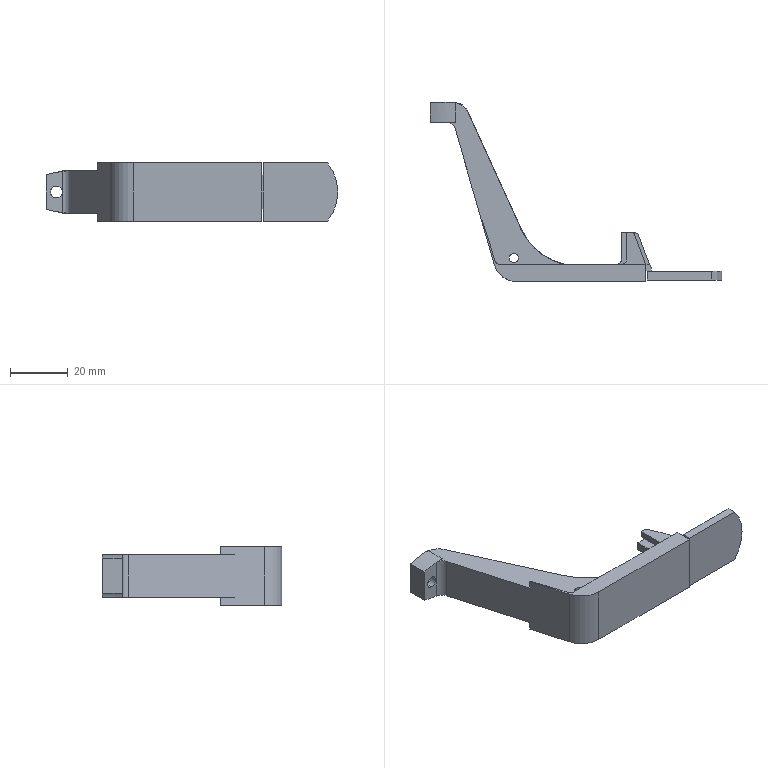Part | SolidWorks | features BaseBody 1 | 1 solid | 139 faces | box 100.61 x 62 x 20.1 mm | volume 11692 mm3 | plane 69 | cylinder 45 | torus 19 | spline 6 | commonest cylinder face diameters 0.2 x8 0.4 x8 4 x8 3.2 x6 2 x2 3 x2